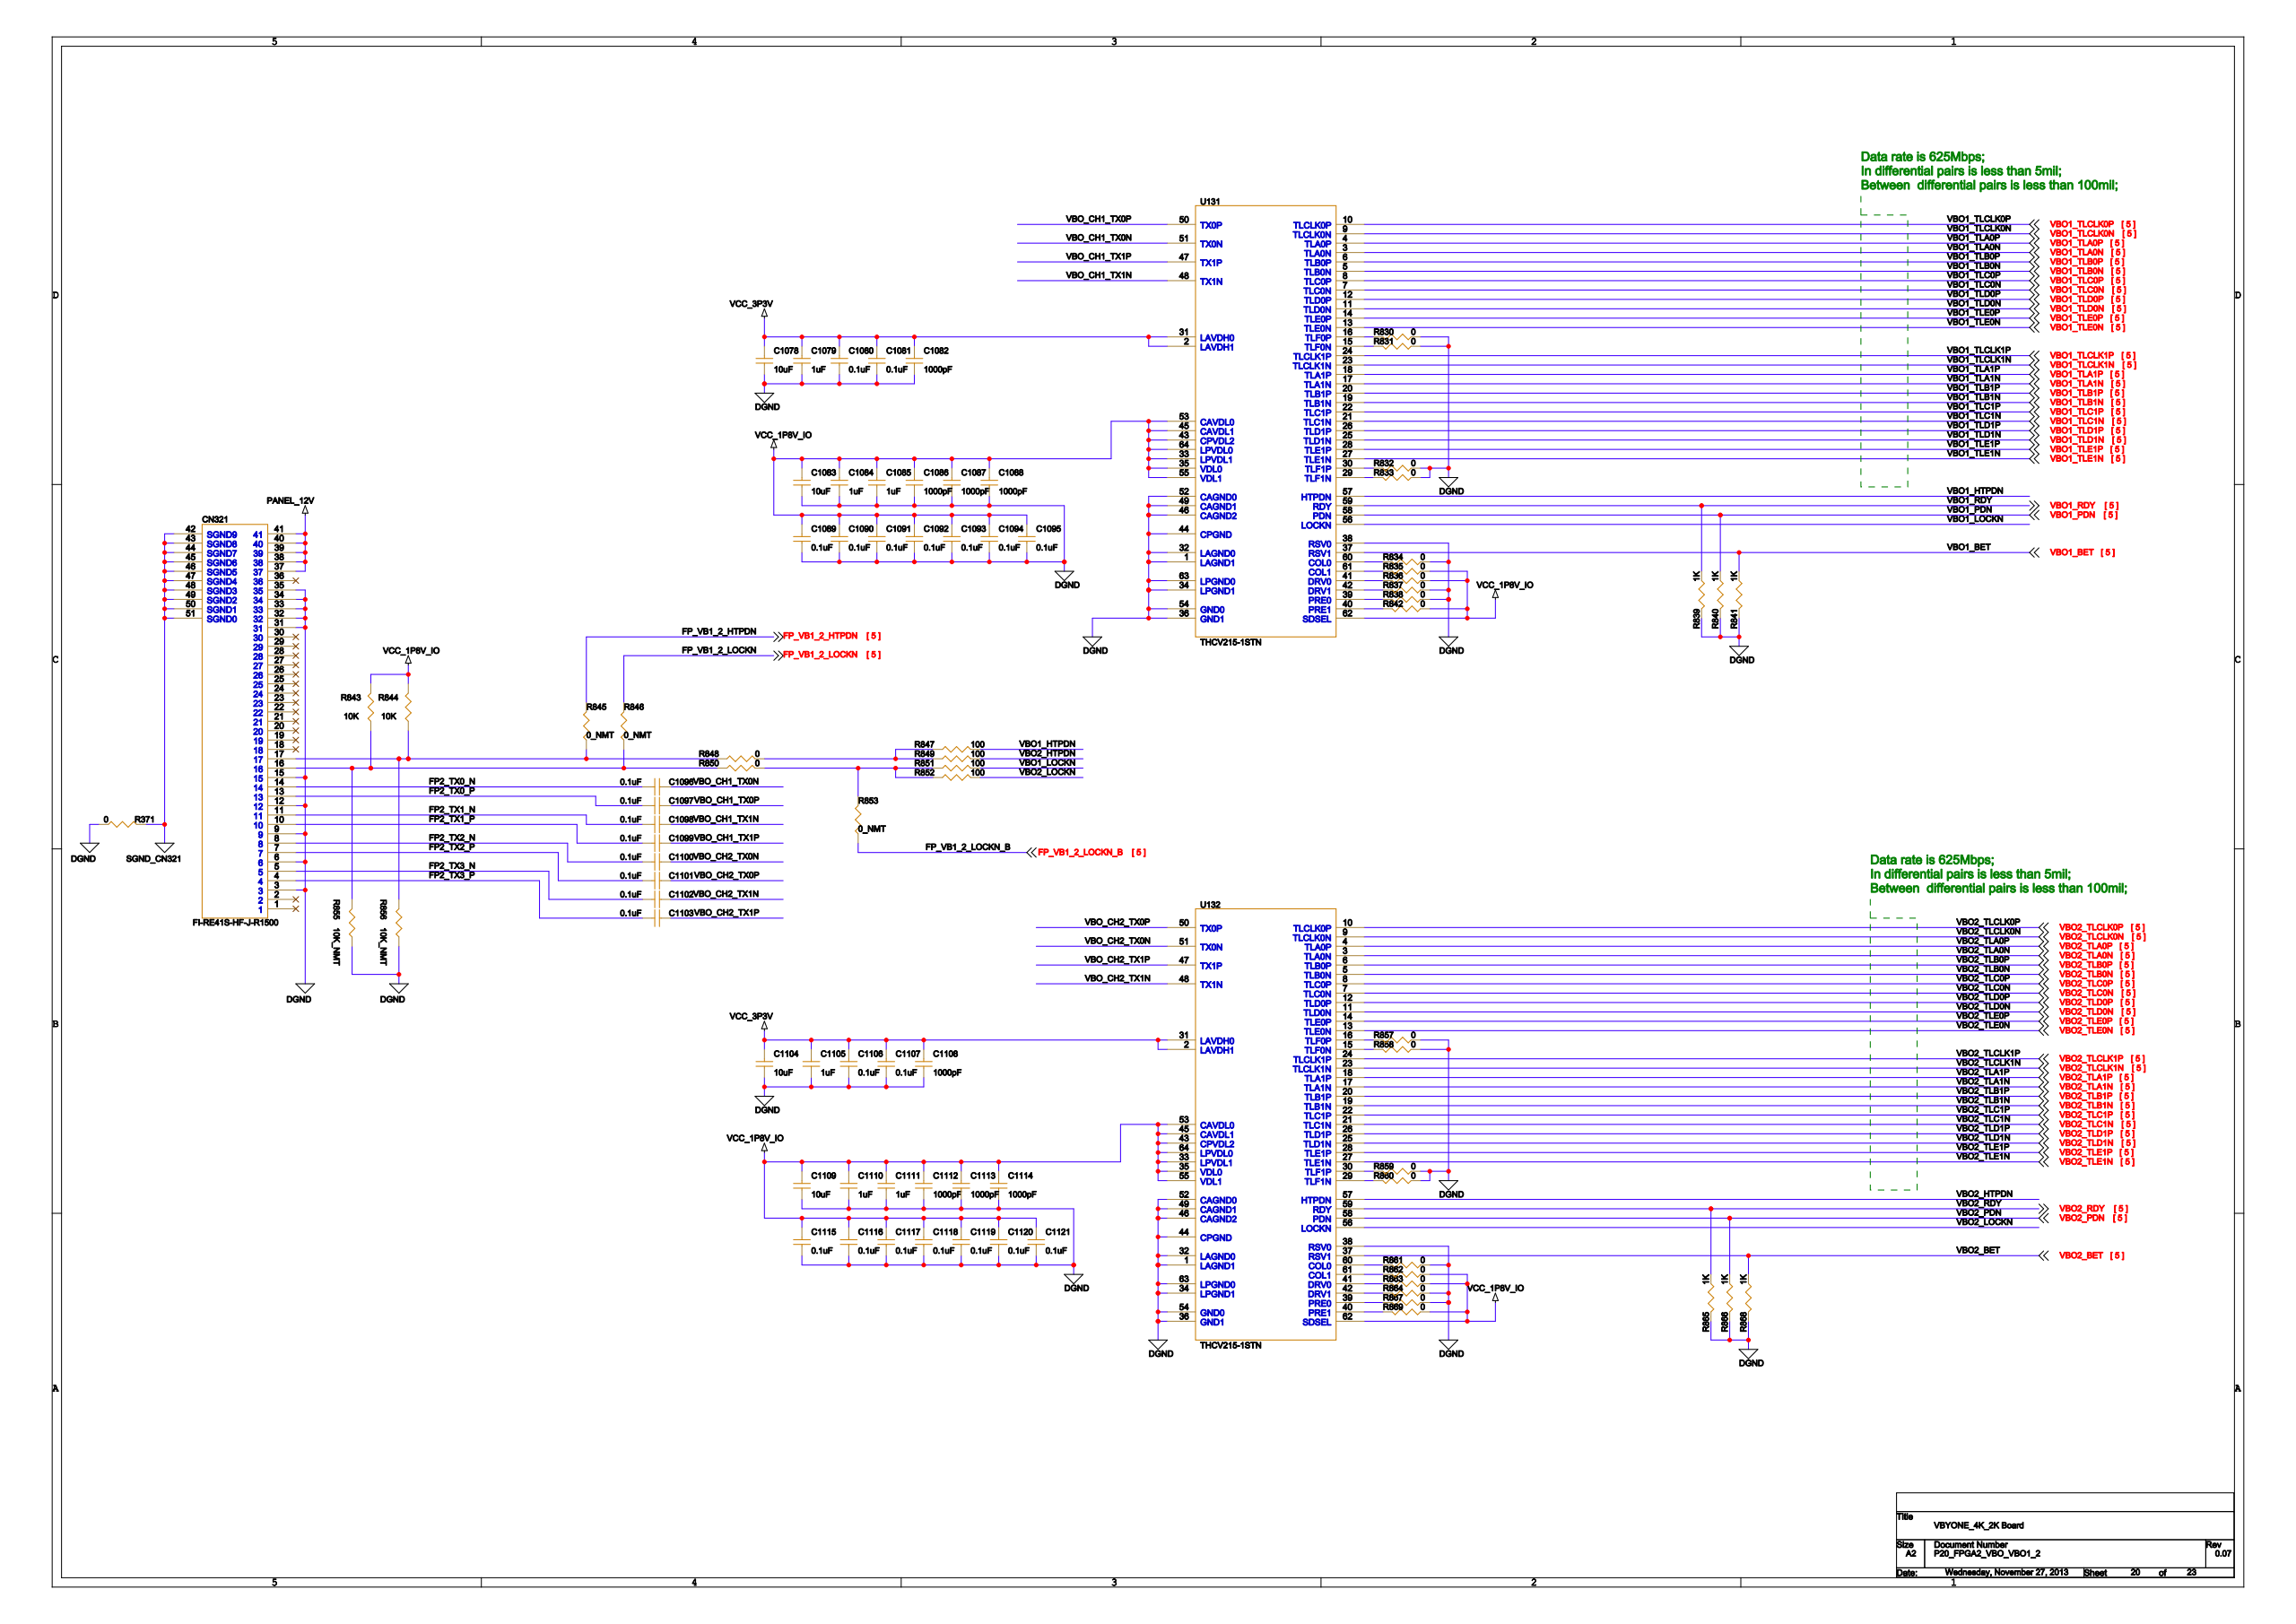Circuit board | Cadence Allegro | 1712 parts | 1495 nets | one sheet of the schematic
Parts on this sheet (reference | value | footprint):
C1078 | 10uF | CRC2012RZAS
C1079 | 1uF | CRC1608RZAS
C1080 | 0.1uF | CRC1005RZAS
C1081 | 0.1uF | CRC1005RZAS
C1082 | 1000pF | CRC1608RZAS
C1083 | 10uF | CRC2012RZAS
C1084 | 1uF | CRC1608RZAS
C1085 | 1uF | CRC1608RZAS
C1086 | 1000pF | CRC1608RZAS
C1087 | 1000pF | CRC1608RZAS
C1088 | 1000pF | CRC1608RZAS
C1089 | 0.1uF | CRC1005RZAS
C1090 | 0.1uF | CRC1005RZAS
C1091 | 0.1uF | CRC1005RZAS
C1092 | 0.1uF | CRC1005RZAS
C1093 | 0.1uF | CRC1005RZAS
C1094 | 0.1uF | CRC1005RZAS
C1095 | 0.1uF | CRC1005RZAS
C1096 | 0.1uF | CRC1005RZAS
C1097 | 0.1uF | CRC1005RZAS
C1098 | 0.1uF | CRC1005RZAS
C1099 | 0.1uF | CRC1005RZAS
C1100 | 0.1uF | CRC1005RZAS
C1101 | 0.1uF | CRC1005RZAS
C1102 | 0.1uF | CRC1005RZAS
C1103 | 0.1uF | CRC1005RZAS
C1104 | 10uF | CRC2012RZAS
C1105 | 1uF | CRC1608RZAS
C1106 | 0.1uF | CRC1005RZAS
C1107 | 0.1uF | CRC1005RZAS
C1108 | 1000pF | CRC1608RZAS
C1109 | 10uF | CRC2012RZAS
C1110 | 1uF | CRC1608RZAS
C1111 | 1uF | CRC1608RZAS
C1112 | 1000pF | CRC1608RZAS
C1113 | 1000pF | CRC1608RZAS
C1114 | 1000pF | CRC1608RZAS
C1115 | 0.1uF | CRC1005RZAS
C1116 | 0.1uF | CRC1005RZAS
C1117 | 0.1uF | CRC1005RZAS
C1118 | 0.1uF | CRC1005RZAS
C1119 | 0.1uF | CRC1005RZAS
C1120 | 0.1uF | CRC1005RZAS
C1121 | 0.1uF | CRC1005RZAS
CN321 | FI-RE41S-HF-J-R1500 | CAC041RCAS
R371 | 0 | CRC1608RZAS
R830 | 0 | CRC1608RZAS
R831 | 0 | CRC1608RZAS
R832 | 0 | CRC1608RZAS
R833 | 0 | CRC1608RZAS
R834 | 0 | CRC1608RZAS
R835 | 0 | CRC1608RZAS
R836 | 0 | CRC1608RZAS
R837 | 0 | CRC1608RZAS
R838 | 0 | CRC1608RZAS
R839 | 1K | CRC1608RZAS
R840 | 1K | CRC1608RZAS
R841 | 1K | CRC1608RZAS
R842 | 0 | CRC1608RZAS
R843 | 10K | CRC1005RZAS
R844 | 10K | CRC1005RZAS
R845 | 0_NMT | CRC1608RZAS
R846 | 0_NMT | CRC1608RZAS
R847 | 100 | CRC1005RZAS
R848 | 0 | CRC1608RZAS
R849 | 100 | CRC1005RZAS
R850 | 0 | CRC1608RZAS
R851 | 100 | CRC1005RZAS
R852 | 100 | CRC1005RZAS
R853 | 0_NMT | CRC1608RZAS
R855 | 10K_NMT | CRC1005RZAS
R856 | 10K_NMT | CRC1005RZAS
R857 | 0 | CRC1608RZAS
R858 | 0 | CRC1608RZAS
R859 | 0 | CRC1608RZAS
R860 | 0 | CRC1608RZAS
R861 | 0 | CRC1608RZAS
R862 | 0 | CRC1608RZAS
R863 | 0 | CRC1608RZAS
R864 | 0 | CRC1608RZAS
R865 | 1K | CRC1608RZAS
R866 | 1K | CRC1608RZAS
R867 | 0 | CRC1608RZAS
R868 | 1K | CRC1608RZAS
R869 | 0 | CRC1608RZAS
U131 | THCV215-1STN | SOC064RCAT
U132 | THCV215-1STN | SOC064RCAT
Nets of these parts (net: part-pin ...):
VCC_3P3V: C1078-2 C1079-2 C1080-2 C1081-2 C1082-2 C1104-2 C1105-2 C1106-2 C1107-2 C1108-2 U131-2 U131-31 U132-2 U132-31
DGND: C1078-1 C1079-1 C1080-1 C1081-1 C1082-1 C1083-1 C1084-1 C1085-1 C1086-1 C1087-1 C1088-1 C1089-1 C1090-1 C1091-1 C1092-1 C1093-1 C1094-1 C1095-1 C1104-1 C1105-1 C1106-1 C1107-1 C1108-1 C1109-1 C1110-1 C1111-1 C1112-1 C1113-1 C1114-1 C1115-1 C1116-1 C1117-1 C1118-1 C1119-1 C1120-1 C1121-1 R371-2 R830-2 R831-2 R832-2 R833-2 R834-2 R837-2 R838-2 R839-1 R840-1 R841-1 R855-2 R856-2 R857-2 R858-2 R859-2 R860-2 R861-2 R864-2 R865-1 R866-1 R867-2 R868-1 CN321-3 CN321-6 CN321-9 CN321-12 CN321-15 CN321-31 CN321-32 CN321-33 CN321-34 CN321-35 U131-1 U131-32 U131-34 U131-36 U131-38 U131-44 U131-46 U131-49 U131-52 U131-54 U131-63 U132-1 U132-32 U132-34 U132-36 U132-38 U132-44 U132-46 U132-49 U132-52 U132-54 U132-63
VCC_1P8V_IO: C1083-2 C1084-2 C1085-2 C1086-2 C1087-2 C1088-2 C1089-2 C1090-2 C1091-2 C1092-2 C1093-2 C1094-2 C1095-2 C1109-2 C1110-2 C1111-2 C1112-2 C1113-2 C1114-2 C1115-2 C1116-2 C1117-2 C1118-2 C1119-2 C1120-2 C1121-2 R835-2 R836-2 R842-2 R843-1 R844-1 R862-2 R863-2 R869-2 U131-33 U131-35 U131-43 U131-45 U131-53 U131-55 U131-62 U131-64 U132-33 U132-35 U132-43 U132-45 U132-53 U132-55 U132-62 U132-64
VBO_CH1_TX0N: C1096-1 U131-51
FP2_TX0_N: C1096-2 CN321-14
VBO_CH1_TX0P: C1097-1 U131-50
FP2_TX0_P: C1097-2 CN321-13
VBO_CH1_TX1N: C1098-1 U131-48
FP2_TX1_N: C1098-2 CN321-11
VBO_CH1_TX1P: C1099-1 U131-47
FP2_TX1_P: C1099-2 CN321-10
VBO_CH2_TX0N: C1100-1 U132-51
FP2_TX2_N: C1100-2 CN321-8
VBO_CH2_TX0P: C1101-1 U132-50
FP2_TX2_P: C1101-2 CN321-7
VBO_CH2_TX1N: C1102-1 U132-48
FP2_TX3_N: C1102-2 CN321-5
VBO_CH2_TX1P: C1103-1 U132-47
FP2_TX3_P: C1103-2 CN321-4
PANEL_12V: CN321-37 CN321-38 CN321-39 CN321-40 CN321-41
SGND_CN321: R371-1 CN321-42 CN321-43 CN321-44 CN321-45 CN321-46 CN321-47 CN321-48 CN321-49 CN321-50 CN321-51
N19761851: R843-2 R846-2 R850-2 R855-1 CN321-16
N19761847: R844-2 R845-2 R848-2 R856-1 CN321-17
N19761983: R847-2 R848-1 R849-2
N19761985: R850-1 R851-2 R852-2 R853-1
FP_VB1_2_HTPDN: R845-1
FP_VB1_2_LOCKN: R846-1
FP_VB1_2_LOCKN_B: R853-2
VBO1_HTPDN: R847-1 U131-57
VBO2_HTPDN: R849-1 U132-57
VBO1_LOCKN: R851-1 U131-56
VBO2_LOCKN: R852-1 U132-56
VBO1_RDY: R839-2 U131-59
VBO1_PDN: R840-2 U131-58
VBO1_BET: R841-2 U131-37
VBO2_RDY: R865-2 U132-59
VBO2_PDN: R866-2 U132-58
VBO2_BET: R868-2 U132-37
N19760692: R830-1 U131-16
N19913343: R831-1 U131-15
N19931554: R832-1 U131-30
N19931555: R833-1 U131-29
N20033527: R834-1 U131-60
N20033841: R835-1 U131-61
N19760495: R836-1 U131-41
N19760493: R837-1 U131-42
N19760501: R838-1 U131-39
N19760505: R842-1 U131-40
N19922857: R857-1 U132-16
N19922847: R858-1 U132-15
N19930963: R859-1 U132-30
N19930962: R860-1 U132-29
N20034393: R861-1 U132-60
N20034589: R862-1 U132-61
N19914119: R863-1 U132-41
N19914117: R864-1 U132-42
N19914133: R867-1 U132-39
N19914135: R869-1 U132-40
VBO2_TLE1P: U132-28
VBO2_TLE1N: U132-27
VBO1_TLD1P: U131-26
VBO1_TLD1N: U131-25
VBO2_TLA1P: U132-18
VBO2_TLD1P: U132-26
VBO1_TLCLK1P: U131-24
VBO1_TLCLK1N: U131-23
VBO1_TLB0P: U131-6
VBO2_TLA1N: U132-17
VBO2_TLD1N: U132-25
VBO2_TLCLK1P: U132-24
VBO1_TLA0P: U131-4
VBO1_TLB0N: U131-5
VBO2_TLC1P: U132-22
VBO2_TLCLK1N: U132-23
VBO1_TLA0N: U131-3
VBO1_TLD0P: U131-12
VBO1_TLC0P: U131-8
VBO2_TLC1N: U132-21
VBO2_TLB1P: U132-20
VBO1_TLD0N: U131-11
VBO1_TLC0N: U131-7
VBO2_TLD0P: U132-12
VBO2_TLB1N: U132-19
VBO1_TLA1P: U131-18
VBO1_TLA1N: U131-17
VBO2_TLD0N: U132-11
VBO1_TLC1P: U131-22
VBO1_TLB1P: U131-20
VBO1_TLB1N: U131-19
VBO2_TLC0P: U132-8
VBO2_TLC0N: U132-7
VBO1_TLC1N: U131-21
VBO1_TLCLK0P: U131-10
VBO2_TLE0P: U132-14
VBO2_TLE0N: U132-13
VBO2_TLCLK0P: U132-10
VBO1_TLCLK0N: U131-9
VBO2_TLB0P: U132-6
VBO2_TLA0P: U132-4
VBO2_TLCLK0N: U132-9
VBO1_TLE0P: U131-14
VBO1_TLE0N: U131-13
VBO2_TLB0N: U132-5
VBO2_TLA0N: U132-3
VBO1_TLE1P: U131-28
VBO1_TLE1N: U131-27